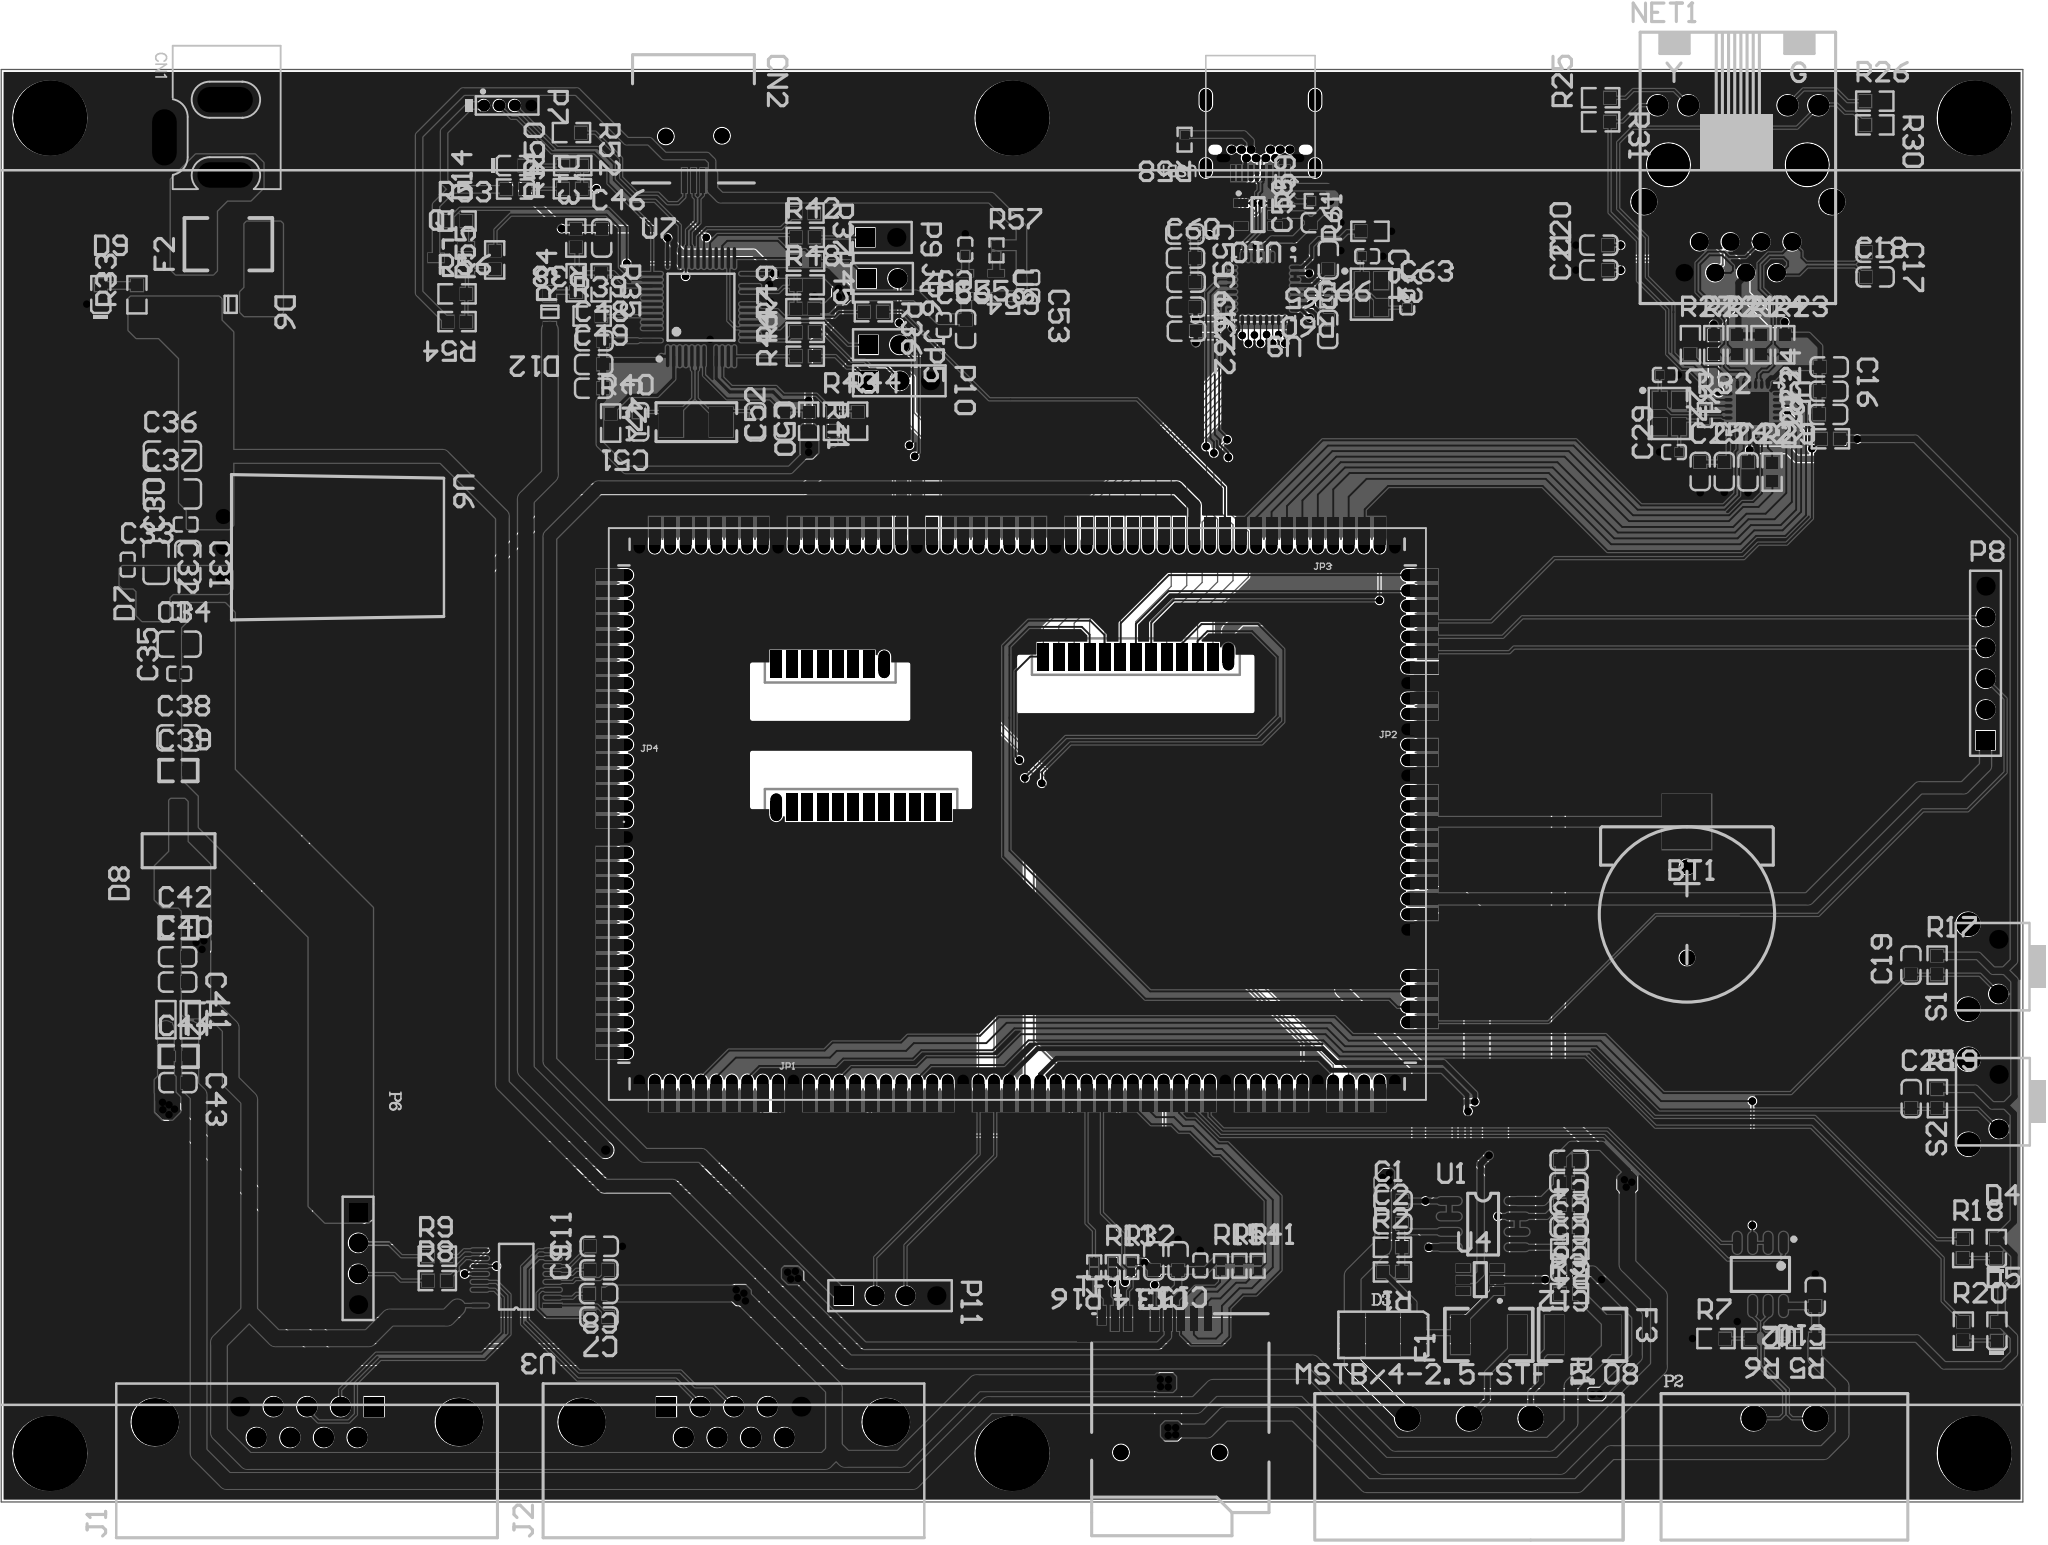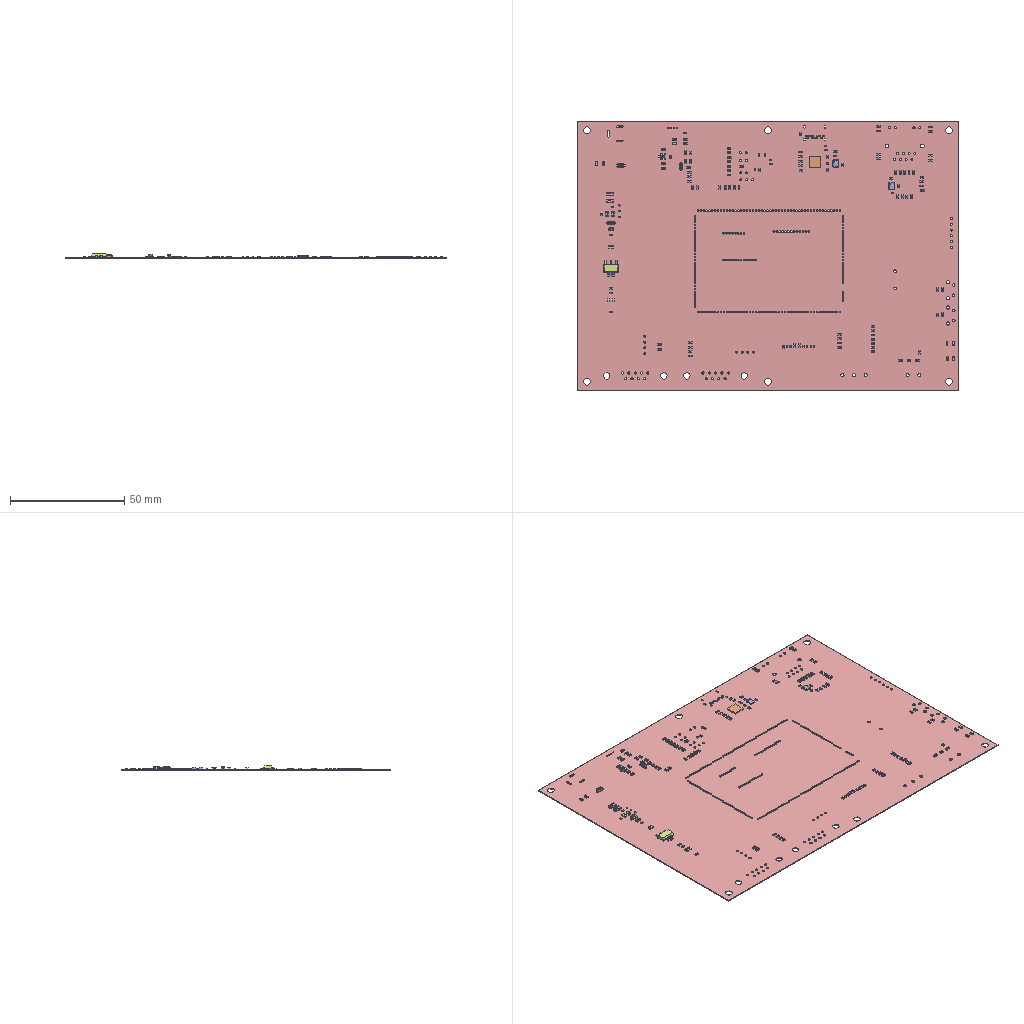Circuit board layout | Altium Designer | box 166.5 x 118 x 2 mm
Layer stack:
# Altium Designer layer stack of 11 (unit mm; dielectric type: 0 none, 1 core, 2 prepreg, 3 surface material)
index,name,kind,layer,copper_thickness_mm,dielectric_type,dielectric_thickness_mm,dielectric_material,dielectric_constant
0,Top Paste,other,,,,,,
1,Top Overlay,other,,,,,,
2,Top Solder,dielectric,,,3,0.0102,Solder Resist,3.5
3,Top Layer,copper,Top Layer,0.0356,,,,
4,Dielectric1,dielectric,,,0,0.32,FR-4,4.8
5,Bottom Layer,copper,Bottom Layer,0.0356,,,,
6,Bottom Solder,dielectric,,,3,0.0102,Solder Resist,3.5
7,Bottom Overlay,other,,,,,,
8,Bottom Paste,other,,,,,,
# drill layer pairs: low layer,high layer
drill_pair,Top Layer,Bottom Layer
Part placement:
Designator,Comment,Layer,Footprint,Center-X(mm),Center-Y(mm),Rotation
U4,SRV05-4-P-T7,TopLayer,SOT-23-6,126.06,17.704,0
F3,SMD1812P050TF/30,TopLayer,1812,134.48,13.157,360
C12,10uF,10V,TopLayer,0603_C,133.426,18.39,180
C1,100pF,50V,TopLayer,0603_C,118.872,24.206,0
JP2,Header 32,TopLayer,SIP-32-1.27-SMD-H-R,120.859,57.325,180
JP4,Header 32,TopLayer,SIP-32-1.27-SMD-H,54.959,56.054,180
JP3,Header 50,TopLayer,SIP-50-1.27-SMD-H,87.909,78.844,90
JP1,Header 50,TopLayer,SIP-50-1.27-SMD-H-R,87.909,33.264,90
P5,Header 8,BottomLayer,CN8SM,72.517,68.393,180
P3,Header 13,BottomLayer,CN13SM,97.688,69.028,180
P4,Header 12,BottomLayer,CN12SM,75.057,56.617,360
BT1,CR2032-3V,TopLayer,BT1,143.075,47.787,90
C54,10uF,TopLayer,0402_C,88.748,100.254,180
C42,0.1uF,TopLayer,0603,18.834,46.685,360
C39,0.1uF,TopLayer,0603,18.834,59.639,360
C7,0.1uF,TopLayer,0603_C,53.467,14.63,180
C57,0.1uF,TopLayer,0402_C,83.642,102.565,270
C8,0.1uF,TopLayer,0603_C,53.442,16.561,180
C19,10nF,TopLayer,0603_C,161.519,43.612,90
C9,0.1uF,TopLayer,0603_C,53.467,18.517,180
C64,20pF,TopLayer,0402_C,116.738,102.006,360
C10,100nF,TopLayer,0603_C,153.645,16.307,270
C11,0.1uF,TopLayer,0603_C,53.492,20.447,180
C13,22uF,6.3V,TopLayer,0603_C,101.168,19.253,270
C14,22uF,6.3V,TopLayer,0603_C,99.162,19.253,270
C15,100nF,TopLayer,0402_C,102.997,18.872,270
C28,10nF,TopLayer,0603_C,161.544,32.614,90
C16,22nF,TopLayer,0603_C,154.788,92.888,360
C17,10pF,TopLayer,0603_C,158.572,102.337,360
C18,10pF,TopLayer,0603_C,158.572,100.305,360
C56,10uF, 6.3V,TopLayer,0402_C,81.864,96.342,90
C20,10pF,TopLayer,0603_C,135.814,102.921,180
C21,10pF,TopLayer,0603_C,135.814,100.863,180
C22,100nF,TopLayer,0603_C,148.107,84.252,90
C23,100nF,TopLayer,0603_C,154.737,88.976,180
C24,100nF,TopLayer,0603_C,154.762,90.881,180
C25,10uF,TopLayer,0603_C,144.17,84.277,90
C36,10uF,50V,TopLayer,1206_C,18.339,85.547,360
C37,10uF,50V,TopLayer,1206_C,18.339,82.423,360
C30,0.1uF,TopLayer,0402_C,19.431,79.908,180
C31,22uF,25V,TopLayer,0805_C,19.609,76.784,270
C32,22uF,25V,TopLayer,0805_C,16.993,76.784,270
C33,0.1uF,TopLayer,0402_C,14.656,76.606,90
C26,100nF,TopLayer,0603_C,146.152,84.277,90
C35,0.1uF,TopLayer,0402_C,18.898,67.615,180
C27,20pF,TopLayer,0402_C,141.249,92.227,360
C29,20pF,TopLayer,0402_C,142.011,85.877,180
C34,22uF,25V,TopLayer,0805_C,18.898,70.053,0
C38,22uF,25V,TopLayer,0805_C,18.872,62.332,360
C40,22uF,6.3V,TopLayer,0603_C,18.771,44.298,360
C41,22uF,6.3V,TopLayer,0603_C,18.771,42.215,360
C43,22uF,6.3V,TopLayer,0603_C,18.796,33.934,360
C44,0.1uF,TopLayer,0603,18.86,36.093,360
C51,20pF,TopLayer,0603_C,56.744,88.367,270
C53,0.1uF,TopLayer,0402_C,88.748,98.704,360
C58,100nF,TopLayer,0603_C,112.878,104.775,180
C59,100nF,TopLayer,0603_C,101.727,103.835,360
C60,100nF,TopLayer,0603_C,101.778,101.854,360
C61,100nF,TopLayer,0603_C,101.829,99.873,360
C62,100nF,TopLayer,0603_C,101.854,95.834,360
C63,20pF,TopLayer,0402_C,120.04,98.196,90
C65,100nF,TopLayer,0603_C,113.538,101.702,270
C66,100nF,TopLayer,0603_C,113.487,95.987,90
C67,100nF,TopLayer,0603_C,101.829,97.815,360
CN2,MiniUSB,TopLayer,Mini-USB-AB,61.278,111.608,270
D7,B5819W  SL,TopLayer,SOD-123,18.847,72.771,180
D4,green LED 0603,TopLayer,0603_LED_S1,168.554,20.258,90
D5,red LED 0603,TopLayer,0603_LED_S1,168.605,13.454,90
D6,B5819W  SL,TopLayer,SOD-123,23.139,98.044,360
D9,RED,TopLayer,0603_LED_S1,12.446,98.831,90
D12,B5819W  SL,TopLayer,SOD-123,49.428,97.434,270
D13,red LED 0603,TopLayer,0603_LED_S1,46.558,109.474,360
D8,CL1117-3.3,TopLayer,SOT-223,18.847,53.035,90
D14,green LED 0603,TopLayer,0603_LED_S1,46.609,107.544,180
F2,SMD1812P050TF/30,TopLayer,1812,22.949,102.997,180
J1,DB9F,TopLayer,DB9RA/F,29.413,5.969,180
J2,DB9M,TopLayer,DB9RA/M,64.567,5.969,180
L1,4.7uH ±10%,TopLayer,0603_L,19.812,39.116,270
L2,4.7uH ±10%,TopLayer,0603_L,17.805,39.116,270
R5,360Ω,TopLayer,0603_R,152.832,12.852,180
R6,120Ω,TopLayer,0603_R,149.149,12.852,180
R54,10K,TopLayer,0603_R,41.783,96.622,180
R60,1MΩ,TopLayer,0402_R,113.462,98.781,270
R7,360Ω,TopLayer,0603_R,145.466,12.852,360
R56,36K,TopLayer,0603_R,41.783,98.908,360
R8,100Ω,TopLayer,0603_R,40.157,17.628,0
R9,100Ω,TopLayer,0603_R,40.157,19.634,360
R58,5K1,TopLayer,0402_R,101.702,111.608,270
R59,5K1,TopLayer,0402_R,112.573,106.553,180
R17,10K,TopLayer,0603_R,163.678,43.612,90
R11,47K,TopLayer,0402_R,107.721,18.847,90
R12,47K,TopLayer,0402_R,97.307,18.745,90
R13,47K,TopLayer,0402_R,95.783,18.745,90
R14,47K,TopLayer,0402_R,106.223,18.847,90
R15,47K,TopLayer,0402_R,104.699,18.821,90
R16,100Ω,TopLayer,0402_R,94.259,18.72,270
R18,680Ω,TopLayer,0603_R,165.786,20.269,90
R19,10K,TopLayer,0603_R,163.703,32.614,90
R20,680Ω,TopLayer,0603_R,165.837,13.462,90
R21,49.9Ω,TopLayer,0603_R,147.218,94.717,90
R22,49.9Ω,TopLayer,0603_R,145.288,94.717,90
R23,49.9Ω,TopLayer,0603_R,151.13,94.717,90
R24,49.9Ω,TopLayer,0603_R,149.174,94.717,90
R25,510Ω,TopLayer,0603_R,135.966,115.062,180
R26,510Ω,TopLayer,0603_R,158.547,114.783,360
R27,12.1KΩ,TopLayer,0603_R,143.358,94.717,90
R28,10KΩ,TopLayer,0603_R,154.889,86.97,180
R29,510Ω,TopLayer,0603_R,150.089,84.226,90
R30,10KΩ,TopLayer,0603_R,158.547,112.827,360
R31,10KΩ,TopLayer,0603_R,135.966,113.081,360
R32,1M,TopLayer,0402_R,144.551,88.925,90
R50,510Ω,TopLayer,0603_R,51.308,109.474,180
R51,510Ω,TopLayer,0603_R,51.283,107.569,180
R57,10K,TopLayer,0402_R,86.208,102.489,90
R61,12KΩ,TopLayer,0603_R,116.967,104.064,180
R33,10K,TopLayer,0603_R,15.418,98.831,90
S1,F1,TopLayer,Reset_TE,167.468,43.485,90
S2,F1,TopLayer,Reset_TE,167.493,32.36,90
TF1,TF,TopLayer,MICROSD,101.16,9.374,0
U3,SP3232EEY-L/TR,TopLayer,TSSOP-16,46.657,17.845,180
U1,LM358,TopLayer,SO-8,126.289,22.276,0
U2,SP3485EN-L/TR,TopLayer,SOIC-8_150mil,149.123,18.136,180
U6,ZY7805LS-1000,TopLayer,ZY78xxLS-1000,22.504,78.029,270
U9,USB330,TopLayer,QFN-32_5x5x05P,108.204,99.339,180
U10,TPD4E001DBVR,TopLayer,SOT-23-6,107.747,105.435,180
Y1,25MHz 12PF,TopLayer,SMD-3225_4P,141.63,89.052,270
Y2,8MHz,TopLayer,SMD-5032_2P,61.493,88.341,180
Y3,24MHz,TopLayer,SMD-3225_4P,117.094,98.882,270
USB1,USB_TypeC_Receptacle,TopLayer,USB_TYPEC,107.95,111.862,180
C2,100pF,50V,TopLayer,0603_C,118.847,22.301,0
C3,10uF,10V,TopLayer,0603_C,133.35,25.705,180
C4,100nF,50V,TopLayer,0603_C,133.375,27.534,180
C6,100pF,50V,TopLayer,0603_C,133.375,22.047,180
F1,SMD1812P050TF/30,TopLayer,1812,126.759,13.157,180
P1,SENSOR,TopLayer,5.08*3B,125.12,6.283,360
R3,1MΩ,TopLayer,0603_R,133.401,16.561,0
R4,100KΩ,TopLayer,0603_R,133.426,20.218,180
R1,10KΩ,TopLayer,0603_R,118.821,18.339,180
R2,10KΩ,TopLayer,0603_R,118.821,20.371,360
U5,LAN8720A,TopLayer,QFN-24_4X4x05P,148.488,89.433,270
C52,100nF,TopLayer,0603_C,68.732,88.417,90
C5,100pF,50V,TopLayer,0603_C,133.375,23.876,180
R41,100K,TopLayer,0603_R,70.739,88.417,270
C49,100nF,TopLayer,0603_C,53.035,93.091,360
C50,20pF,TopLayer,0603_C,66.37,88.367,270
C48,100nF,TopLayer,0603_C,53.061,95.047,0
C47,100nF,TopLayer,0603_C,53.035,91.135,360
R39,100K,TopLayer,0603_R,52.908,97.079,0
R35,4K7,TopLayer,0603_R,53.645,99.822,270
R34,2K7,TopLayer,0603_R,51.587,99.822,90
R53,1K5,TopLayer,0603_R,41.783,104.902,360
R55,100,TopLayer,0603_R,44.882,101.702,90
R48,[N/A],TopLayer,0603_R,70.46,99.644,0
R36,100,TopLayer,0603_R,76.073,97.434,360
R43,4K7,TopLayer,0603_R,72.782,88.408,90
R45,100,TopLayer,0603_R,70.485,101.6,360
R37,100,TopLayer,0603_R,70.434,105.562,360
R38,10K,TopLayer,0603_R,51.562,103.505,270
R40,10K,TopLayer,0603_R,54.432,88.265,90
R42,100,TopLayer,0603_R,70.46,103.556,0
R44,4K7,TopLayer,0603_R,74.778,88.417,90
R46,100,TopLayer,0603_R,70.46,93.777,180
R47,100,TopLayer,0603_R,70.46,95.733,180
R49,[N/A],TopLayer,0603_R,70.434,97.688,180
C55,0.1uF,25V,TopLayer,0603_C,83.668,96.012,90
Q1,SS8050 Y1,TopLayer,SOT-23(SOT-23-3),41.3,101.879,360
R52,100KΩ,TopLayer,0603_R,51.206,112.192,360
U7,STM32F103CBT6,TopLayer,LQFP-48_7x7x05P,61.874,97.815,0
JP5,,TopLayer,HDR1X2,76.937,94.717,360
JP6,,TopLayer,HDR1X2,76.784,100.178,360
P6,UART7,TopLayer,HDR1X4,33.63,19.456,270
D3,P6SMB6.8CA,TopLayer,P6KESMD,118.045,13.157,360
CN1,DC-10B,TopLayer,DC10B,20.69,111.8,270
NET1,HR911105A,TopLayer,RJ45,147.269,107.546,0
P7,STLK_SWD,TopLayer,127*4,45.917,114.427,360
P2,RS485,TopLayer,508*2B,151.105,6.283,360
C46,100nF,TopLayer,0603_C,53.696,103.505,90
U8,SP6205-3.3,TopLayer,SOT23-5,84.912,99.659,270
P8,SPI2,TopLayer,HDR1X6,167.665,68.478,90
P9,MCO,TopLayer,HDR1X2,76.683,103.556,360
P10,UART1,TopLayer,HDR1X3,78.207,91.745,360
P11,TSWD,TopLayer,HDR1X4,77.445,16.383,360
Pad and via stacks, first 77 of 95 lines:
# Altium Designer via and pad stacks of 11 (unit mm). Each distinct definition once, with the count of objects using it.
# via: kind,start_layer,end_layer,hole_mm,diameter_mm,mode(0 simple;1 top-mid-bottom;2 full stack),diameter_per_layer,count,example_net
# pad: kind,layer,hole_mm,hole_type(0 round;1 square;2 slot),plating,top_size,top_shape(1 round;2 rect;3 octagon;9 rounded rect),mid_size,bottom_size,mode,footprint,size_per_layer,count,example
pad,Multi-Layer,1.4,0,plated,2x2,1,2x2,2x2,0,5.08*3B,,3,P1.1
pad,Multi-Layer,0.9,0,plated,1.5x1.5,2,1.5x1.5,1.5x1.5,0,HDR1X2,,3,P9.1
pad,Multi-Layer,0.9,0,plated,1.5x1.5,1,1.5x1.5,1.5x1.5,0,HDR1X2,,3,P9.2
pad,Multi-Layer,0.9,0,plated,1.5x1.5,2,1.5x1.5,1.5x1.5,0,HDR1X3,,1,P10.1
pad,Multi-Layer,0.9,0,plated,1.5x1.5,1,1.5x1.5,1.5x1.5,0,HDR1X3,,2,P10.2
pad,Multi-Layer,0.9,0,plated,1.5x1.5,1,1.5x1.5,1.5x1.5,0,HDR1X4,,6,P11.4
pad,Multi-Layer,0.9,0,plated,1.5x1.5,2,1.5x1.5,1.5x1.5,0,HDR1X4,,2,P11.1
pad,Multi-Layer,3,0,plated,6x6,1,6x6,6x6,0,,,6,0
pad,Multi-Layer,0.9,0,plated,1.5x1.5,2,1.5x1.5,1.5x1.5,0,HDR1X6,,1,P8.1
pad,Multi-Layer,0.9,0,plated,1.5x1.5,1,1.5x1.5,1.5x1.5,0,HDR1X6,,5,P8.2
pad,Multi-Layer,1.2,0,plated,1.2x1.2,1,1.2x1.2,1.2x1.2,0,BT1,,2,BT1.0
pad,Multi-Layer,1.4,0,plated,2x2,1,2x2,2x2,0,508*2B,,2,P2.1
pad,Multi-Layer,0.5,0,plated,0.9x0.9,1,0.9x0.9,0.9x0.9,0,127*4,,4,P7.4
pad,Multi-Layer,1.016,0,plated,1.651x1.651,1,1.651x1.651,1.651x1.651,0,RJ45,,4,NET1.12
pad,Multi-Layer,1.63,0,plated,2.05x2.05,1,2.05x2.05,2.05x2.05,0,RJ45,,2,NET1.0
pad,Multi-Layer,0.89,0,plated,1.397x1.397,1,1.397x1.397,1.397x1.397,0,RJ45,,8,NET1.1
pad,Multi-Layer,0.762,0,plated,1.143x1.143,1,1.143x1.143,1.143x1.143,0,DC10B,,12,CN1.3
pad,Multi-Layer,0.762,0,plated,2.032x4.572,1,2.032x4.572,2.032x4.572,0,DC10B,,2,CN1.1
pad,Multi-Layer,0.762,0,plated,4.572x2.032,1,4.572x2.032,4.572x2.032,0,DC10B,,1,CN1.2
pad,Multi-Layer,0.4,0,plated,0.64x0.64,1,0.64x0.64,0.64x0.64,0,USB_TYPEC,,4,USB1.B5
pad,Multi-Layer,0.4,0,plated,0.65x0.65,1,0.65x0.65,0.65x0.65,0,USB_TYPEC,,6,USB1.B8
pad,Multi-Layer,0.4,2,plated,1.14x0.64,1,1.14x0.64,1.14x0.64,0,USB_TYPEC,,2,USB1.B1
pad,Multi-Layer,0.5,2,plated,1.8x1,1,1.8x1,1.8x1,0,USB_TYPEC,,2,USB1.0
pad,Multi-Layer,0.64,2,unplated,0.64x0,1,0.64x0,0.64x0,0,USB_TYPEC,,2,USB1.0
pad,Multi-Layer,0.5,2,plated,1.6x1,1,1.6x1,1.6x1,0,USB_TYPEC,,2,USB1.0
pad,Multi-Layer,0.65,0,plated,1.2x1.2,1,1.2x1.2,1.2x1.2,0,ZY78xxLS-1000,,3,U6.3
pad,Multi-Layer,1.4,0,plated,1.9x1.9,1,1.9x1.9,1.9x1.9,0,Reset_TE,,4,S1.0
pad,Multi-Layer,1.1,0,plated,1.5x1.5,1,1.5x1.5,1.5x1.5,0,Reset_TE,,4,S1.1
pad,Multi-Layer,0.9652,0,plated,1.575x1.575,2,1.575x1.575,1.575x1.575,0,DB9RA/F,,1,J1.1
pad,Multi-Layer,0.9652,0,plated,1.575x1.575,1,1.575x1.575,1.575x1.575,0,DB9RA/F,,8,J1.2
pad,Multi-Layer,2.794,0,plated,3.81x3.81,1,3.81x3.81,3.81x3.81,0,DB9RA/F,,2,J1.
pad,Multi-Layer,0.9652,0,plated,1.575x1.575,2,1.575x1.575,1.575x1.575,0,DB9RA/M,,1,J2.1
pad,Multi-Layer,0.9652,0,plated,1.575x1.575,1,1.575x1.575,1.575x1.575,0,DB9RA/M,,8,J2.2
pad,Multi-Layer,2.794,0,plated,3.81x3.81,1,3.81x3.81,3.81x3.81,0,DB9RA/M,,2,J2.
pad,Multi-Layer,0,0,plated,2.25x0.95,2,2.25x0.95,2.25x0.95,0,CN8SM,,7,P5.8
pad,Multi-Layer,0,0,plated,2.25x0.95,1,2.25x0.95,2.25x0.95,0,CN8SM,,1,P5.1
pad,Multi-Layer,0.8,0,plated,1x0.95,2,1x0.95,1x0.95,0,CN8SM,,8,P5.6
pad,Multi-Layer,0.8,0,plated,1x0.95,2,1x0.95,1x0.95,0,CN12SM,,12,P4.12
pad,Multi-Layer,0,0,plated,2.25x0.95,2,2.25x0.95,2.25x0.95,0,CN12SM,,11,P4.8
pad,Multi-Layer,0,0,plated,2.25x0.95,1,2.25x0.95,2.25x0.95,0,CN12SM,,1,P4.1
pad,Multi-Layer,0,0,plated,2.25x0.95,2,2.25x0.95,2.25x0.95,0,CN13SM,,12,P3.13
pad,Multi-Layer,0,0,plated,2.25x0.95,1,2.25x0.95,2.25x0.95,0,CN13SM,,1,P3.1
pad,Multi-Layer,0.8,0,plated,1x0.95,2,1x0.95,1x0.95,0,CN13SM,,13,P3.12
pad,Multi-Layer,0.7,0,plated,1.5x0.95,1,1.5x0.95,1.5x0.95,0,SIP-32-1.27-SMD-H,,32,JP4.5
pad,Multi-Layer,0.7,0,plated,1.5x0.95,1,1.5x0.95,1.5x0.95,0,SIP-32-1.27-SMD-H-R,,28,JP2.5
pad,Multi-Layer,0.7,0,plated,1.5x0.95,1,1.5x0.95,1.5x0.95,0,SIP-50-1.27-SMD-H,,50,JP3.5
pad,Multi-Layer,0.7,0,plated,1.5x0.95,1,1.5x0.95,1.5x0.95,0,SIP-50-1.27-SMD-H-R,,50,JP1.5
pad,Top Layer,0,0,plated,0.93x0.98,2,0.93x0.98,0.93x0.98,0,0603_R,,98,R33.2
pad,Top Layer,0,0,plated,4.5x4,2,4.5x4,4.5x4,0,BT1,,2,BT1.1
pad,Top Layer,0,0,plated,0.93x0.98,2,0.93x0.98,0.93x0.98,0,0603_C,,90,C46.2
pad,Top Layer,0,0,plated,0.508x1.27,2,0.508x1.27,0.508x1.27,0,SOT23-5,,5,U8.1
pad,Top Layer,0,0,plated,1.5x0.3,2,1.5x0.3,1.5x0.3,0,TSSOP-16,,1,U3.1
pad,Top Layer,0,0,plated,1.5x0.3,1,1.5x0.3,1.5x0.3,0,TSSOP-16,,15,U3.2
pad,Top Layer,0,0,plated,0.93x0.98,2,0.93x0.98,0.93x0.98,0,0603_LED_S1,,10,D9.K
pad,Top Layer,0,0,plated,2x3.5,2,2x3.5,2x3.5,0,P6KESMD,,2,D3.2
pad,Top Layer,0,0,plated,0.28x1.8,1,0.28x1.8,0.28x1.8,0,LQFP-48_7x7x05P,,48,U7.1
pad,Top Layer,0,0,plated,0.7x1.25,2,0.7x1.25,0.7x1.25,0,SOT-23(SOT-23-3),,3,Q1.3
pad,Top Layer,0,0,plated,0.28x0.7,1,0.28x0.7,0.28x0.7,0,QFN-24_4X4x05P,,24,U5.1
pad,Top Layer,0,0,plated,2.68x2.68,2,2.68x2.68,2.68x2.68,0,QFN-24_4X4x05P,,1,U5.0
pad,Top Layer,0,0,plated,1.524x3.175,2,1.524x3.175,1.524x3.175,0,1812,,6,F1.1
pad,Top Layer,0,0,plated,1.3x0.3,2,1.3x0.3,1.3x0.3,0,USB_TYPEC,,12,USB1.A1
pad,Top Layer,0,0,plated,3.2x3.2,2,3.2x3.2,3.2x3.2,0,QFN-32_5x5x05P,,1,U9.33
pad,Top Layer,0,0,plated,0.28x0.85,1,0.28x0.85,0.28x0.85,0,QFN-32_5x5x05P,,32,U9.32
pad,Top Layer,0,0,plated,0.6x0.65,2,0.6x0.65,0.6x0.65,0,0402_R,,22,R58.2
pad,Top Layer,0,0,plated,0.6x0.65,2,0.6x0.65,0.6x0.65,0,0402_C,,24,C63.2
pad,Top Layer,0,0,plated,1.4x1.15,2,1.4x1.15,1.4x1.15,0,SMD-3225_4P,,8,Y3.2
pad,Top Layer,0,0,plated,0.6x1.1,2,0.6x1.1,0.6x1.1,0,SOT-23-6,,12,U10.6
pad,Top Layer,0,0,plated,1.25x1,2,1.25x1,1.25x1,0,SOD-123,,6,D12.2
pad,Top Layer,0,0,plated,2.4x1.9,2,2.4x1.9,2.4x1.9,0,SMD-5032_2P,,2,Y2.2
pad,Top Layer,0,0,plated,2.032x2.032,2,2.032x2.032,2.032x2.032,0,Mini-USB-AB,,4,CN2.0
pad,Top Layer,0,0,plated,2.032x0.381,2,2.032x0.381,2.032x0.381,0,Mini-USB-AB,,5,CN2.5
pad,Top Layer,0,0,plated,1.16x1.47,2,1.16x1.47,1.16x1.47,0,0805_C,,8,C34.1
pad,Top Layer,0,0,plated,1.13x1.8,2,1.13x1.8,1.13x1.8,0,1206_C,,4,C37.2
pad,Top Layer,0,0,plated,3.5x2.2,2,3.5x2.2,3.5x2.2,0,SOT-223,,1,D8.2
Copper pours:
name,layer,net,type(0 solid;1 hatched;2 none)
Top Layer-No Net,Top Layer,GND,0
Top Layer-No Net,Top Layer,AGND,0
Top Layer-No Net,Top Layer,AGND,0
Top Layer-No Net,Top Layer,AGND,0
Top Layer-No Net,Top Layer,3V3,0
Top Layer-No Net,Top Layer,3V3,0
Top Layer-No Net,Top Layer,3V3,0
Top Layer-No Net,Top Layer,3V3,0
Top Layer-No Net,Top Layer,A3V3,0
Top Layer-No Net,Top Layer,NetC31_2,0
Top Layer-No Net,Top Layer,AIN2,0
Top Layer-No Net,Top Layer,NetD6_1,0
Top Layer-No Net,Top Layer,NetCN1_1,0
TopLayer-No Net,Top Layer,+3V3_ST_LINK,0
TopLayer-No Net,Top Layer,+3V3_ST_LINK,0
TopLayer-No Net,Top Layer,+5V,0
TopLayer-No Net,Top Layer,3V3,0
Top Layer-No Net,Bottom Layer,GND,0
Top Layer-No Net,Bottom Layer,AGND,0
Top Layer-No Net,Bottom Layer,AGND,0
Top Layer-No Net,Bottom Layer,AGND,0
Top Layer-No Net,Bottom Layer,3V3,0
Top Layer-No Net,Bottom Layer,3V3,0
Top Layer-No Net,Bottom Layer,3V3,0
Top Layer-No Net,Bottom Layer,A3V3,0
TopLayer-No Net,Bottom Layer,+3V3_ST_LINK,0
TopLayer-No Net,Bottom Layer,+3V3_ST_LINK,0
Design rules, without the lines most boards share:
# Altium Designer design rules of 11 (exported by Altium Designer, unit mm)
# columns: name | kind | enabled | priority | scope1 | scope2 | descriptor | typed fields (field=value)
Schematic Matched Net Lengths_8 | 4 | enabled | 1 | InNet('TD_N') | All | Matched Lengths(Tolerance=100mil) (InNet('TD_N')) |
Schematic Matched Net Lengths_6 | 4 | enabled | 3 | InNet('TD_N') | All | Matched Lengths(Tolerance=100mil) (InNet('TD_N')) |
Schematic Matched Net Lengths_5 | 4 | enabled | 4 | InNet('TD_P') | All | Matched Lengths(Tolerance=100mil) (InNet('TD_P')) |
Schematic Matched Net Lengths_2 | 4 | enabled | 7 | InNet('TD_N') | All | Matched Lengths(Tolerance=100mil) (InNet('TD_N')) |
Schematic Matched Net Lengths_1 | 4 | enabled | 8 | InNet('RD_P') | All | Matched Lengths(Tolerance=100mil) (InNet('RD_P')) |
Schematic Matched Net Lengths | 4 | enabled | 9 | InNet('RD_N') | All | Matched Lengths(Tolerance=100mil) (InNet('RD_N')) |
SilkToSilkClearance | 55 | enabled | 1 | All | All | Silk to Silk (Clearance=0mil) (All),(All) |
SilkToSolderMaskClearance | 54 | disabled | 1 | IsPad | All | Silk To Solder Mask (Clearance=0mil) (Disabled)(IsPad),(All) |
MinimumSolderMaskSliver | 53 | enabled | 1 | All | All | Minimum Solder Mask Sliver (Gap=0mil) (All),(All) |
HoleToHoleClearance | 52 | enabled | 1 | All | All | Hole To Hole Clearance (Gap=10mil) (All),(All) | gap=0.254
DiffPairsRouting | 51 | enabled | 1 | All | All | Differential Pairs Uncoupled Length using the Gap Constraints (Min=6mil) (Max=6mil) (Prefered=6mil)  and Width Constraints (Min=15mil) (Max=15mil) (Prefered=15mil) (All) |
Fanout_BGA | 49 | disabled | 4 | All | All | Fanout Control Rule ( (Disabled)(All) ) |
Fanout_LCC | 49 | disabled | 5 | All | All | Fanout Control Rule ( (Disabled)(All) ) |
Fanout_SOIC | 49 | disabled | 3 | All | All | Fanout Control Rule ( (Disabled)(All) ) |
Fanout_Small | 49 | disabled | 1 | All | All | Fanout Control Rule ( (Disabled)(All) ) |
Fanout_Default | 49 | enabled | 2 | All | All | Fanout Control Rule ( (All) ) |
ComponentClearance | 24 | enabled | 1 | All | All | Component Clearance Constraint ( Horizontal Gap = 10mil, Vertical Gap = 0mil ) (All),(All)  | gap=0.254
SolderMaskExpansion | 13 | enabled | 1 | All | All | Solder Mask Expansion (Expansion =4mil) (All) | expansion=0.1016
PasteMaskExpansion | 14 | enabled | 1 | All | All | Paste Mask Expansion (Expansion =0mil) (All) | expansion=0
RoutingVias | 11 | enabled | 1 | All | All | Routing Via (MinHoleWidth=12mil) (MaxHoleWidth=12mil) (PreferredHoleWidth=12mil) (MinWidth=24mil) (MaxWidth=24mil) (PreferedWidth=24mil) (All) | via_min_hole=0.3048 via_max_hole=0.3048 via_preferred_diameter=0.6096 via_preferred_hole=0.3048
Width | 2 | enabled | 1 | All | All | Width Constraint (Min=4mil) (Max=80mil) (Preferred=6mil) (All) |
PolygonConnect | 20 | enabled | 1 | All | All | Polygon Connect Rule(Direct Connect )(Conductor Width=10mil) (Relief Angle=90 Angle) (Entries=4) (Air Gap Width=10mil) (All),(All) | connect_style(0=relief,1=direct,2=none)=1 relief_conductor_width=0.254 relief_entries=4
PlaneConnect | 6 | enabled | 1 | All | All | Power Plane Connect Rule(Relief Connect )(Expansion=20mil) (Conductor Width=10mil) (Air Gap=10mil) (Entries=4) (All) | relief_conductor_width=0.254 relief_entries=4 relief_expansion=0.508
Clearance | 0 | enabled | 1 | All | All | Clearance Constraint (Gap=4mil) (All),(All) | gap=0.1016
Schematic Matched Net Lengths_3 | 4 | enabled | 6 | InNet('TD_N') | All | Matched Lengths(Tolerance=100mil) (InNet('TD_N')) |
Schematic Matched Net Lengths_4 | 4 | enabled | 5 | InNet('TD_P') | All | Matched Lengths(Tolerance=100mil) (InNet('TD_P')) |
Schematic Matched Net Lengths_7 | 4 | enabled | 2 | InNet('TD_N') | All | Matched Lengths(Tolerance=100mil) (InNet('TD_N')) |
Classes set for this board:
# Altium Designer classes of 11 (member kind: 0 net, 1 component, 2 from-to, 3 pad, 4 layer, 5 differential pair, 6 design channel, 7 polygon, 8 structure, 9 xSignal)
# columns: class name | member kind | superclass | members
USB | 1 | no | C65; C66; C67; USB1; Y3; C60; C63; R61; R58; U10; C64; C59; C62; R60; R59; C58; C61; U9;
ST_Link | 1 | no | CN2; JP5; JP6; Q1; Y2; C56; R48; R49; R50; R51; R52; R53; R54; R55; C51; R57; C47; D13; R48; R55; R56; C57; R54; R38; R46; C53; R53; R50; C52; C56; D14; R43; R40; R47; D12; R51; C50; R45; R42; R49; C48; C49; C54; C55; Q1; R34; R35; R36; R37; R39; R41; R44; R52; U7; JP5; JP6; P7; C46; U8; P9; P10;
PWR | 1 | no | BT1; D9; L1; L2; C40; C34; C41; C42; C35; C38; C43; U6; C44; C39; C30; D7; C31; C32; C33; C36; C37; D6; D8; F2; R33; CN1;
Ethernet | 1 | no | Y1; C29; C17; C22; R21; C23; C26; R22; U5; C16; C20; C24; C18; C21; C25; C27; R23; R24; R25; R26; R27; R28; R29; R30; R31; R32; NET1;
Core | 1 | no | C19; C28; JP1; JP2; JP3; JP4; P3; P4; P5; S1; S2; R18; D5; R17; R19; D4; R20; P8; P11;
Connect | 1 | no | J1; J2; P6; TF1; U3; R11; U2; C15; R12; R16; R13; C8; C9; C13; R5; R7; R9; R14; C7; C10; C11; C14; R6; R8; R15; P2;
ADC_Exp | 1 | no | C5; D3; R1; R2; R3; R4; U1; F1; P1; C4; R3; C5; R1; R2; C3; R4; C2; C6; C1; C12; F3; U4;